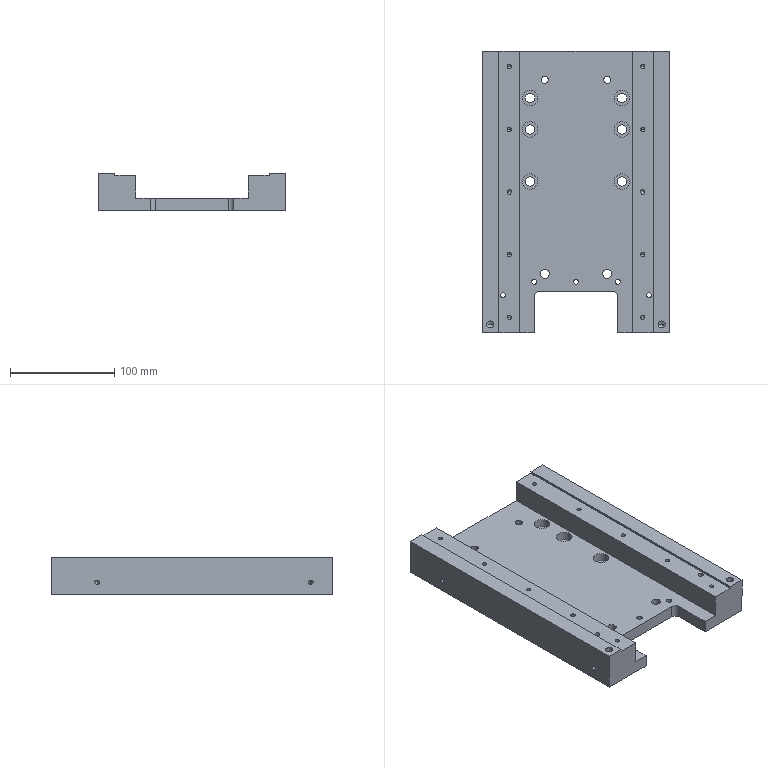Part | SolidWorks | features HoleWzd 11, ICE 2, Cut 1, Extrusion 1, Fillet 1 | 1 solid | 168 faces | box 180 x 270 x 36 mm | volume 970158 mm3 | cylinder 94 | cone 50 | plane 24 | commonest cylinder face diameters 4.2 x34 3.3 x12 9 x12 15 x12 5 x10 6.8 x8